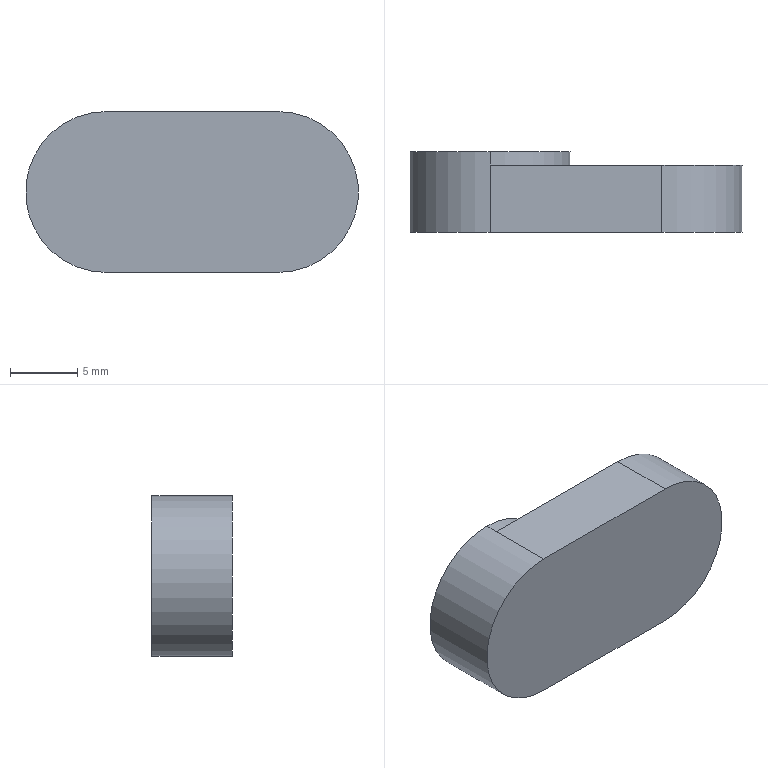Part | STEP file | JTJTRUYIU_Default | 1 solid | 8 faces | box 24.8 x 6 x 12 mm | volume 1447 mm3 | plane 5 | cylinder 3 | commonest cylinder face diameters 12 x3
STEP:
#1=CARTESIAN_POINT('',(0.,0.,0.));
#2=DIRECTION('',(0.,0.,1.));
#3=DIRECTION('',(1.,0.,0.));
#4=AXIS2_PLACEMENT_3D('',#1,#2,#3);
#5=CARTESIAN_POINT('',(-6.4,6.,6.));
#6=VERTEX_POINT('',#5);
#7=CARTESIAN_POINT('',(-6.4,6.,-6.));
#8=VERTEX_POINT('',#7);
#9=CARTESIAN_POINT('',(-6.4,6.,0.));
#10=DIRECTION('',(0.,1.,0.));
#11=DIRECTION('',(0.,0.,1.));
#12=AXIS2_PLACEMENT_3D('',#9,#10,#11);
#13=CIRCLE('',#12,6.);
#14=CARTESIAN_POINT('',(-6.4,5.,0.));
#15=DIRECTION('',(0.,-1.,0.));
#16=DIRECTION('',(0.,0.,-1.));
#17=AXIS2_PLACEMENT_3D('',#14,#15,#16);
#18=CYLINDRICAL_SURFACE('',#17,6.);
#19=CARTESIAN_POINT('',(3.142,-1.));
#20=DIRECTION('',(-1.,0.));
#21=VECTOR('',#20,1.);
#22=LINE('',#19,#21);
#23=(GEOMETRIC_REPRESENTATION_CONTEXT(2)PARAMETRIC_REPRESENTATION_CONTEXT()REPRESENTATION_CONTEXT('',''));
#24=DEFINITIONAL_REPRESENTATION('',(#22),#23);
#25=PCURVE('',#18,#24);
#26=CARTESIAN_POINT('',(-6.4,6.,0.));
#27=DIRECTION('',(0.,1.,0.));
#28=DIRECTION('',(0.,0.,1.));
#29=AXIS2_PLACEMENT_3D('',#26,#27,#28);
#30=PLANE('',#29);
#31=CARTESIAN_POINT('',(0.,0.));
#32=DIRECTION('',(1.,0.));
#33=AXIS2_PLACEMENT_2D('',#31,#32);
#34=CIRCLE('',#33,6.);
#35=(GEOMETRIC_REPRESENTATION_CONTEXT(2)PARAMETRIC_REPRESENTATION_CONTEXT()REPRESENTATION_CONTEXT('',''));
#36=DEFINITIONAL_REPRESENTATION('',(#34),#35);
#37=PCURVE('',#30,#36);
#38=SURFACE_CURVE('',#13,(#25,#37),.PCURVE_S1.);
#39=EDGE_CURVE('',#6,#8,#38,.T.);
#40=ORIENTED_EDGE('',*,*,#39,.F.);
#41=CARTESIAN_POINT('',(-6.4,5.,6.));
#42=VERTEX_POINT('',#41);
#43=CARTESIAN_POINT('',(-6.4,5.,6.));
#44=DIRECTION('',(0.,-1.,0.));
#45=VECTOR('',#44,1.);
#46=LINE('',#43,#45);
#47=CARTESIAN_POINT('',(3.142,0.));
#48=DIRECTION('',(0.,1.));
#49=VECTOR('',#48,1.);
#50=LINE('',#47,#49);
#51=(GEOMETRIC_REPRESENTATION_CONTEXT(2)PARAMETRIC_REPRESENTATION_CONTEXT()REPRESENTATION_CONTEXT('',''));
#52=DEFINITIONAL_REPRESENTATION('',(#50),#51);
#53=PCURVE('',#18,#52);
#54=CARTESIAN_POINT('',(-6.4,5.,0.));
#55=DIRECTION('',(0.,-1.,0.));
#56=DIRECTION('',(0.,0.,-1.));
#57=AXIS2_PLACEMENT_3D('',#54,#55,#56);
#58=CYLINDRICAL_SURFACE('',#57,6.);
#59=CARTESIAN_POINT('',(3.142,0.));
#60=DIRECTION('',(0.,1.));
#61=VECTOR('',#60,1.);
#62=LINE('',#59,#61);
#63=(GEOMETRIC_REPRESENTATION_CONTEXT(2)PARAMETRIC_REPRESENTATION_CONTEXT()REPRESENTATION_CONTEXT('',''));
#64=DEFINITIONAL_REPRESENTATION('',(#62),#63);
#65=PCURVE('',#58,#64);
#66=SURFACE_CURVE('',#46,(#53,#65),.PCURVE_S1.);
#67=EDGE_CURVE('',#6,#42,#66,.T.);
#68=ORIENTED_EDGE('',*,*,#67,.T.);
#69=CARTESIAN_POINT('',(-6.4,5.,-6.));
#70=VERTEX_POINT('',#69);
#71=CARTESIAN_POINT('',(-6.4,5.,0.));
#72=DIRECTION('',(0.,1.,0.));
#73=DIRECTION('',(0.,0.,1.));
#74=AXIS2_PLACEMENT_3D('',#71,#72,#73);
#75=CIRCLE('',#74,6.);
#76=CARTESIAN_POINT('',(3.142,0.));
#77=DIRECTION('',(-1.,0.));
#78=VECTOR('',#77,1.);
#79=LINE('',#76,#78);
#80=(GEOMETRIC_REPRESENTATION_CONTEXT(2)PARAMETRIC_REPRESENTATION_CONTEXT()REPRESENTATION_CONTEXT('',''));
#81=DEFINITIONAL_REPRESENTATION('',(#79),#80);
#82=PCURVE('',#18,#81);
#83=CARTESIAN_POINT('',(6.4,5.,0.));
#84=DIRECTION('',(0.,1.,0.));
#85=DIRECTION('',(0.,0.,1.));
#86=AXIS2_PLACEMENT_3D('',#83,#84,#85);
#87=PLANE('',#86);
#88=CARTESIAN_POINT('',(0.,-12.8));
#89=DIRECTION('',(1.,0.));
#90=AXIS2_PLACEMENT_2D('',#88,#89);
#91=CIRCLE('',#90,6.);
#92=(GEOMETRIC_REPRESENTATION_CONTEXT(2)PARAMETRIC_REPRESENTATION_CONTEXT()REPRESENTATION_CONTEXT('',''));
#93=DEFINITIONAL_REPRESENTATION('',(#91),#92);
#94=PCURVE('',#87,#93);
#95=SURFACE_CURVE('',#75,(#82,#94),.PCURVE_S1.);
#96=EDGE_CURVE('',#42,#70,#95,.T.);
#97=ORIENTED_EDGE('',*,*,#96,.T.);
#98=CARTESIAN_POINT('',(-6.4,5.,-6.));
#99=DIRECTION('',(0.,-1.,0.));
#100=VECTOR('',#99,1.);
#101=LINE('',#98,#100);
#102=CARTESIAN_POINT('',(0.,0.));
#103=DIRECTION('',(0.,1.));
#104=VECTOR('',#103,1.);
#105=LINE('',#102,#104);
#106=(GEOMETRIC_REPRESENTATION_CONTEXT(2)PARAMETRIC_REPRESENTATION_CONTEXT()REPRESENTATION_CONTEXT('',''));
#107=DEFINITIONAL_REPRESENTATION('',(#105),#106);
#108=PCURVE('',#18,#107);
#109=CARTESIAN_POINT('',(6.283,0.));
#110=DIRECTION('',(0.,1.));
#111=VECTOR('',#110,1.);
#112=LINE('',#109,#111);
#113=(GEOMETRIC_REPRESENTATION_CONTEXT(2)PARAMETRIC_REPRESENTATION_CONTEXT()REPRESENTATION_CONTEXT('',''));
#114=DEFINITIONAL_REPRESENTATION('',(#112),#113);
#115=PCURVE('',#58,#114);
#116=SURFACE_CURVE('',#101,(#108,#115),.PCURVE_S1.);
#117=EDGE_CURVE('',#8,#70,#116,.T.);
#118=ORIENTED_EDGE('',*,*,#117,.F.);
#119=EDGE_LOOP('',(#40,#68,#97,#118));
#120=FACE_BOUND('',#119,.T.);
#121=ADVANCED_FACE('',(#120),#18,.T.);
#122=CARTESIAN_POINT('',(6.4,0.,6.));
#123=VERTEX_POINT('',#122);
#124=CARTESIAN_POINT('',(6.4,0.,-6.));
#125=VERTEX_POINT('',#124);
#126=CARTESIAN_POINT('',(6.4,0.,0.));
#127=DIRECTION('',(0.,1.,0.));
#128=DIRECTION('',(0.,0.,1.));
#129=AXIS2_PLACEMENT_3D('',#126,#127,#128);
#130=CIRCLE('',#129,6.);
#131=CARTESIAN_POINT('',(6.4,5.,0.));
#132=DIRECTION('',(0.,-1.,0.));
#133=DIRECTION('',(0.,0.,-1.));
#134=AXIS2_PLACEMENT_3D('',#131,#132,#133);
#135=CYLINDRICAL_SURFACE('',#134,6.);
#136=CARTESIAN_POINT('',(3.142,5.));
#137=DIRECTION('',(-1.,0.));
#138=VECTOR('',#137,1.);
#139=LINE('',#136,#138);
#140=(GEOMETRIC_REPRESENTATION_CONTEXT(2)PARAMETRIC_REPRESENTATION_CONTEXT()REPRESENTATION_CONTEXT('',''));
#141=DEFINITIONAL_REPRESENTATION('',(#139),#140);
#142=PCURVE('',#135,#141);
#143=CARTESIAN_POINT('',(6.4,0.,0.));
#144=DIRECTION('',(0.,1.,0.));
#145=DIRECTION('',(0.,0.,1.));
#146=AXIS2_PLACEMENT_3D('',#143,#144,#145);
#147=PLANE('',#146);
#148=CARTESIAN_POINT('',(0.,0.));
#149=DIRECTION('',(1.,0.));
#150=AXIS2_PLACEMENT_2D('',#148,#149);
#151=CIRCLE('',#150,6.);
#152=(GEOMETRIC_REPRESENTATION_CONTEXT(2)PARAMETRIC_REPRESENTATION_CONTEXT()REPRESENTATION_CONTEXT('',''));
#153=DEFINITIONAL_REPRESENTATION('',(#151),#152);
#154=PCURVE('',#147,#153);
#155=SURFACE_CURVE('',#130,(#142,#154),.PCURVE_S1.);
#156=EDGE_CURVE('',#123,#125,#155,.T.);
#157=ORIENTED_EDGE('',*,*,#156,.T.);
#158=CARTESIAN_POINT('',(6.4,5.,-6.));
#159=VERTEX_POINT('',#158);
#160=CARTESIAN_POINT('',(6.4,5.,-6.));
#161=DIRECTION('',(0.,-1.,0.));
#162=VECTOR('',#161,1.);
#163=LINE('',#160,#162);
#164=CARTESIAN_POINT('',(0.,0.));
#165=DIRECTION('',(0.,1.));
#166=VECTOR('',#165,1.);
#167=LINE('',#164,#166);
#168=(GEOMETRIC_REPRESENTATION_CONTEXT(2)PARAMETRIC_REPRESENTATION_CONTEXT()REPRESENTATION_CONTEXT('',''));
#169=DEFINITIONAL_REPRESENTATION('',(#167),#168);
#170=PCURVE('',#135,#169);
#171=CARTESIAN_POINT('',(6.4,5.,-6.));
#172=DIRECTION('',(0.,0.,1.));
#173=DIRECTION('',(1.,0.,0.));
#174=AXIS2_PLACEMENT_3D('',#171,#172,#173);
#175=PLANE('',#174);
#176=CARTESIAN_POINT('',(0.,0.));
#177=DIRECTION('',(0.,-1.));
#178=VECTOR('',#177,1.);
#179=LINE('',#176,#178);
#180=(GEOMETRIC_REPRESENTATION_CONTEXT(2)PARAMETRIC_REPRESENTATION_CONTEXT()REPRESENTATION_CONTEXT('',''));
#181=DEFINITIONAL_REPRESENTATION('',(#179),#180);
#182=PCURVE('',#175,#181);
#183=SURFACE_CURVE('',#163,(#170,#182),.PCURVE_S1.);
#184=EDGE_CURVE('',#159,#125,#183,.T.);
#185=ORIENTED_EDGE('',*,*,#184,.F.);
#186=CARTESIAN_POINT('',(6.4,5.,6.));
#187=VERTEX_POINT('',#186);
#188=CARTESIAN_POINT('',(6.4,5.,0.));
#189=DIRECTION('',(0.,1.,0.));
#190=DIRECTION('',(0.,0.,1.));
#191=AXIS2_PLACEMENT_3D('',#188,#189,#190);
#192=CIRCLE('',#191,6.);
#193=CARTESIAN_POINT('',(3.142,0.));
#194=DIRECTION('',(-1.,0.));
#195=VECTOR('',#194,1.);
#196=LINE('',#193,#195);
#197=(GEOMETRIC_REPRESENTATION_CONTEXT(2)PARAMETRIC_REPRESENTATION_CONTEXT()REPRESENTATION_CONTEXT('',''));
#198=DEFINITIONAL_REPRESENTATION('',(#196),#197);
#199=PCURVE('',#135,#198);
#200=CARTESIAN_POINT('',(0.,0.));
#201=DIRECTION('',(1.,0.));
#202=AXIS2_PLACEMENT_2D('',#200,#201);
#203=CIRCLE('',#202,6.);
#204=(GEOMETRIC_REPRESENTATION_CONTEXT(2)PARAMETRIC_REPRESENTATION_CONTEXT()REPRESENTATION_CONTEXT('',''));
#205=DEFINITIONAL_REPRESENTATION('',(#203),#204);
#206=PCURVE('',#87,#205);
#207=SURFACE_CURVE('',#192,(#199,#206),.PCURVE_S1.);
#208=EDGE_CURVE('',#187,#159,#207,.T.);
#209=ORIENTED_EDGE('',*,*,#208,.F.);
#210=CARTESIAN_POINT('',(6.4,5.,6.));
#211=DIRECTION('',(0.,-1.,0.));
#212=VECTOR('',#211,1.);
#213=LINE('',#210,#212);
#214=CARTESIAN_POINT('',(3.142,0.));
#215=DIRECTION('',(0.,1.));
#216=VECTOR('',#215,1.);
#217=LINE('',#214,#216);
#218=(GEOMETRIC_REPRESENTATION_CONTEXT(2)PARAMETRIC_REPRESENTATION_CONTEXT()REPRESENTATION_CONTEXT('',''));
#219=DEFINITIONAL_REPRESENTATION('',(#217),#218);
#220=PCURVE('',#135,#219);
#221=CARTESIAN_POINT('',(6.4,5.,6.));
#222=DIRECTION('',(0.,0.,-1.));
#223=DIRECTION('',(-1.,0.,0.));
#224=AXIS2_PLACEMENT_3D('',#221,#222,#223);
#225=PLANE('',#224);
#226=CARTESIAN_POINT('',(0.,0.));
#227=DIRECTION('',(0.,-1.));
#228=VECTOR('',#227,1.);
#229=LINE('',#226,#228);
#230=(GEOMETRIC_REPRESENTATION_CONTEXT(2)PARAMETRIC_REPRESENTATION_CONTEXT()REPRESENTATION_CONTEXT('',''));
#231=DEFINITIONAL_REPRESENTATION('',(#229),#230);
#232=PCURVE('',#225,#231);
#233=SURFACE_CURVE('',#213,(#220,#232),.PCURVE_S1.);
#234=EDGE_CURVE('',#187,#123,#233,.T.);
#235=ORIENTED_EDGE('',*,*,#234,.T.);
#236=EDGE_LOOP('',(#157,#185,#209,#235));
#237=FACE_BOUND('',#236,.T.);
#238=ADVANCED_FACE('',(#237),#135,.T.);
#239=CARTESIAN_POINT('',(-6.4,0.,-6.));
#240=VERTEX_POINT('',#239);
#241=CARTESIAN_POINT('',(6.4,0.,-6.));
#242=DIRECTION('',(-1.,0.,0.));
#243=VECTOR('',#242,1.);
#244=LINE('',#241,#243);
#245=CARTESIAN_POINT('',(0.,-5.));
#246=DIRECTION('',(-1.,0.));
#247=VECTOR('',#246,1.);
#248=LINE('',#245,#247);
#249=(GEOMETRIC_REPRESENTATION_CONTEXT(2)PARAMETRIC_REPRESENTATION_CONTEXT()REPRESENTATION_CONTEXT('',''));
#250=DEFINITIONAL_REPRESENTATION('',(#248),#249);
#251=PCURVE('',#175,#250);
#252=CARTESIAN_POINT('',(-6.,0.));
#253=DIRECTION('',(0.,-1.));
#254=VECTOR('',#253,1.);
#255=LINE('',#252,#254);
#256=(GEOMETRIC_REPRESENTATION_CONTEXT(2)PARAMETRIC_REPRESENTATION_CONTEXT()REPRESENTATION_CONTEXT('',''));
#257=DEFINITIONAL_REPRESENTATION('',(#255),#256);
#258=PCURVE('',#147,#257);
#259=SURFACE_CURVE('',#244,(#251,#258),.PCURVE_S1.);
#260=EDGE_CURVE('',#125,#240,#259,.T.);
#261=ORIENTED_EDGE('',*,*,#260,.T.);
#262=CARTESIAN_POINT('',(-6.4,5.,-6.));
#263=DIRECTION('',(0.,-1.,0.));
#264=VECTOR('',#263,1.);
#265=LINE('',#262,#264);
#266=CARTESIAN_POINT('',(-12.8,0.));
#267=DIRECTION('',(0.,-1.));
#268=VECTOR('',#267,1.);
#269=LINE('',#266,#268);
#270=(GEOMETRIC_REPRESENTATION_CONTEXT(2)PARAMETRIC_REPRESENTATION_CONTEXT()REPRESENTATION_CONTEXT('',''));
#271=DEFINITIONAL_REPRESENTATION('',(#269),#270);
#272=PCURVE('',#175,#271);
#273=CARTESIAN_POINT('',(6.283,0.));
#274=DIRECTION('',(0.,1.));
#275=VECTOR('',#274,1.);
#276=LINE('',#273,#275);
#277=(GEOMETRIC_REPRESENTATION_CONTEXT(2)PARAMETRIC_REPRESENTATION_CONTEXT()REPRESENTATION_CONTEXT('',''));
#278=DEFINITIONAL_REPRESENTATION('',(#276),#277);
#279=PCURVE('',#58,#278);
#280=SURFACE_CURVE('',#265,(#272,#279),.PCURVE_S1.);
#281=EDGE_CURVE('',#70,#240,#280,.T.);
#282=ORIENTED_EDGE('',*,*,#281,.F.);
#283=CARTESIAN_POINT('',(6.4,5.,-6.));
#284=DIRECTION('',(-1.,0.,0.));
#285=VECTOR('',#284,1.);
#286=LINE('',#283,#285);
#287=CARTESIAN_POINT('',(0.,0.));
#288=DIRECTION('',(-1.,0.));
#289=VECTOR('',#288,1.);
#290=LINE('',#287,#289);
#291=(GEOMETRIC_REPRESENTATION_CONTEXT(2)PARAMETRIC_REPRESENTATION_CONTEXT()REPRESENTATION_CONTEXT('',''));
#292=DEFINITIONAL_REPRESENTATION('',(#290),#291);
#293=PCURVE('',#175,#292);
#294=CARTESIAN_POINT('',(-6.,0.));
#295=DIRECTION('',(0.,-1.));
#296=VECTOR('',#295,1.);
#297=LINE('',#294,#296);
#298=(GEOMETRIC_REPRESENTATION_CONTEXT(2)PARAMETRIC_REPRESENTATION_CONTEXT()REPRESENTATION_CONTEXT('',''));
#299=DEFINITIONAL_REPRESENTATION('',(#297),#298);
#300=PCURVE('',#87,#299);
#301=SURFACE_CURVE('',#286,(#293,#300),.PCURVE_S1.);
#302=EDGE_CURVE('',#159,#70,#301,.T.);
#303=ORIENTED_EDGE('',*,*,#302,.F.);
#304=ORIENTED_EDGE('',*,*,#184,.T.);
#305=EDGE_LOOP('',(#261,#282,#303,#304));
#306=FACE_BOUND('',#305,.T.);
#307=ADVANCED_FACE('',(#306),#175,.F.);
#308=ORIENTED_EDGE('',*,*,#67,.F.);
#309=CARTESIAN_POINT('',(-6.4,6.,0.));
#310=DIRECTION('',(0.,1.,0.));
#311=DIRECTION('',(0.,0.,1.));
#312=AXIS2_PLACEMENT_3D('',#309,#310,#311);
#313=CIRCLE('',#312,6.);
#314=CARTESIAN_POINT('',(9.425,-1.));
#315=DIRECTION('',(-1.,0.));
#316=VECTOR('',#315,1.);
#317=LINE('',#314,#316);
#318=(GEOMETRIC_REPRESENTATION_CONTEXT(2)PARAMETRIC_REPRESENTATION_CONTEXT()REPRESENTATION_CONTEXT('',''));
#319=DEFINITIONAL_REPRESENTATION('',(#317),#318);
#320=PCURVE('',#58,#319);
#321=CARTESIAN_POINT('',(0.,0.));
#322=DIRECTION('',(1.,0.));
#323=AXIS2_PLACEMENT_2D('',#321,#322);
#324=CIRCLE('',#323,6.);
#325=(GEOMETRIC_REPRESENTATION_CONTEXT(2)PARAMETRIC_REPRESENTATION_CONTEXT()REPRESENTATION_CONTEXT('',''));
#326=DEFINITIONAL_REPRESENTATION('',(#324),#325);
#327=PCURVE('',#30,#326);
#328=SURFACE_CURVE('',#313,(#320,#327),.PCURVE_S1.);
#329=EDGE_CURVE('',#8,#6,#328,.T.);
#330=ORIENTED_EDGE('',*,*,#329,.F.);
#331=ORIENTED_EDGE('',*,*,#117,.T.);
#332=ORIENTED_EDGE('',*,*,#281,.T.);
#333=CARTESIAN_POINT('',(-6.4,0.,6.));
#334=VERTEX_POINT('',#333);
#335=CARTESIAN_POINT('',(-6.4,0.,0.));
#336=DIRECTION('',(0.,1.,0.));
#337=DIRECTION('',(0.,0.,1.));
#338=AXIS2_PLACEMENT_3D('',#335,#336,#337);
#339=CIRCLE('',#338,6.);
#340=CARTESIAN_POINT('',(9.425,5.));
#341=DIRECTION('',(-1.,0.));
#342=VECTOR('',#341,1.);
#343=LINE('',#340,#342);
#344=(GEOMETRIC_REPRESENTATION_CONTEXT(2)PARAMETRIC_REPRESENTATION_CONTEXT()REPRESENTATION_CONTEXT('',''));
#345=DEFINITIONAL_REPRESENTATION('',(#343),#344);
#346=PCURVE('',#58,#345);
#347=CARTESIAN_POINT('',(0.,-12.8));
#348=DIRECTION('',(1.,0.));
#349=AXIS2_PLACEMENT_2D('',#347,#348);
#350=CIRCLE('',#349,6.);
#351=(GEOMETRIC_REPRESENTATION_CONTEXT(2)PARAMETRIC_REPRESENTATION_CONTEXT()REPRESENTATION_CONTEXT('',''));
#352=DEFINITIONAL_REPRESENTATION('',(#350),#351);
#353=PCURVE('',#147,#352);
#354=SURFACE_CURVE('',#339,(#346,#353),.PCURVE_S1.);
#355=EDGE_CURVE('',#240,#334,#354,.T.);
#356=ORIENTED_EDGE('',*,*,#355,.T.);
#357=CARTESIAN_POINT('',(-6.4,5.,6.));
#358=DIRECTION('',(0.,-1.,0.));
#359=VECTOR('',#358,1.);
#360=LINE('',#357,#359);
#361=CARTESIAN_POINT('',(3.142,0.));
#362=DIRECTION('',(0.,1.));
#363=VECTOR('',#362,1.);
#364=LINE('',#361,#363);
#365=(GEOMETRIC_REPRESENTATION_CONTEXT(2)PARAMETRIC_REPRESENTATION_CONTEXT()REPRESENTATION_CONTEXT('',''));
#366=DEFINITIONAL_REPRESENTATION('',(#364),#365);
#367=PCURVE('',#58,#366);
#368=CARTESIAN_POINT('',(12.8,0.));
#369=DIRECTION('',(0.,-1.));
#370=VECTOR('',#369,1.);
#371=LINE('',#368,#370);
#372=(GEOMETRIC_REPRESENTATION_CONTEXT(2)PARAMETRIC_REPRESENTATION_CONTEXT()REPRESENTATION_CONTEXT('',''));
#373=DEFINITIONAL_REPRESENTATION('',(#371),#372);
#374=PCURVE('',#225,#373);
#375=SURFACE_CURVE('',#360,(#367,#374),.PCURVE_S1.);
#376=EDGE_CURVE('',#42,#334,#375,.T.);
#377=ORIENTED_EDGE('',*,*,#376,.F.);
#378=EDGE_LOOP('',(#308,#330,#331,#332,#356,#377));
#379=FACE_BOUND('',#378,.T.);
#380=ADVANCED_FACE('',(#379),#58,.T.);
#381=CARTESIAN_POINT('',(6.4,0.,6.));
#382=DIRECTION('',(1.,0.,0.));
#383=VECTOR('',#382,1.);
#384=LINE('',#381,#383);
#385=CARTESIAN_POINT('',(0.,-5.));
#386=DIRECTION('',(-1.,0.));
#387=VECTOR('',#386,1.);
#388=LINE('',#385,#387);
#389=(GEOMETRIC_REPRESENTATION_CONTEXT(2)PARAMETRIC_REPRESENTATION_CONTEXT()REPRESENTATION_CONTEXT('',''));
#390=DEFINITIONAL_REPRESENTATION('',(#388),#389);
#391=PCURVE('',#225,#390);
#392=CARTESIAN_POINT('',(6.,0.));
#393=DIRECTION('',(0.,1.));
#394=VECTOR('',#393,1.);
#395=LINE('',#392,#394);
#396=(GEOMETRIC_REPRESENTATION_CONTEXT(2)PARAMETRIC_REPRESENTATION_CONTEXT()REPRESENTATION_CONTEXT('',''));
#397=DEFINITIONAL_REPRESENTATION('',(#395),#396);
#398=PCURVE('',#147,#397);
#399=SURFACE_CURVE('',#384,(#391,#398),.PCURVE_S1.);
#400=EDGE_CURVE('',#334,#123,#399,.T.);
#401=ORIENTED_EDGE('',*,*,#400,.T.);
#402=ORIENTED_EDGE('',*,*,#234,.F.);
#403=CARTESIAN_POINT('',(6.4,5.,6.));
#404=DIRECTION('',(1.,0.,0.));
#405=VECTOR('',#404,1.);
#406=LINE('',#403,#405);
#407=CARTESIAN_POINT('',(0.,0.));
#408=DIRECTION('',(-1.,0.));
#409=VECTOR('',#408,1.);
#410=LINE('',#407,#409);
#411=(GEOMETRIC_REPRESENTATION_CONTEXT(2)PARAMETRIC_REPRESENTATION_CONTEXT()REPRESENTATION_CONTEXT('',''));
#412=DEFINITIONAL_REPRESENTATION('',(#410),#411);
#413=PCURVE('',#225,#412);
#414=CARTESIAN_POINT('',(6.,0.));
#415=DIRECTION('',(0.,1.));
#416=VECTOR('',#415,1.);
#417=LINE('',#414,#416);
#418=(GEOMETRIC_REPRESENTATION_CONTEXT(2)PARAMETRIC_REPRESENTATION_CONTEXT()REPRESENTATION_CONTEXT('',''));
#419=DEFINITIONAL_REPRESENTATION('',(#417),#418);
#420=PCURVE('',#87,#419);
#421=SURFACE_CURVE('',#406,(#413,#420),.PCURVE_S1.);
#422=EDGE_CURVE('',#42,#187,#421,.T.);
#423=ORIENTED_EDGE('',*,*,#422,.F.);
#424=ORIENTED_EDGE('',*,*,#376,.T.);
#425=EDGE_LOOP('',(#401,#402,#423,#424));
#426=FACE_BOUND('',#425,.T.);
#427=ADVANCED_FACE('',(#426),#225,.F.);
#428=ORIENTED_EDGE('',*,*,#96,.F.);
#429=ORIENTED_EDGE('',*,*,#422,.T.);
#430=ORIENTED_EDGE('',*,*,#208,.T.);
#431=ORIENTED_EDGE('',*,*,#302,.T.);
#432=EDGE_LOOP('',(#428,#429,#430,#431));
#433=FACE_BOUND('',#432,.T.);
#434=ADVANCED_FACE('',(#433),#87,.T.);
#435=ORIENTED_EDGE('',*,*,#156,.F.);
#436=ORIENTED_EDGE('',*,*,#400,.F.);
#437=ORIENTED_EDGE('',*,*,#355,.F.);
#438=ORIENTED_EDGE('',*,*,#260,.F.);
#439=EDGE_LOOP('',(#435,#436,#437,#438));
#440=FACE_BOUND('',#439,.T.);
#441=ADVANCED_FACE('',(#440),#147,.F.);
#442=ORIENTED_EDGE('',*,*,#329,.T.);
#443=ORIENTED_EDGE('',*,*,#39,.T.);
#444=EDGE_LOOP('',(#442,#443));
#445=FACE_BOUND('',#444,.T.);
#446=ADVANCED_FACE('',(#445),#30,.T.);
#447=CLOSED_SHELL('',(#121,#238,#307,#380,#427,#434,#441,#446));
#448=MANIFOLD_SOLID_BREP('',#447);
#449=(LENGTH_UNIT()NAMED_UNIT(*)SI_UNIT(.MILLI.,.METRE.));
#450=UNCERTAINTY_MEASURE_WITH_UNIT(LENGTH_MEASURE(0.0000001),#449,'','');
#451=(NAMED_UNIT(*)PLANE_ANGLE_UNIT()SI_UNIT($,.RADIAN.));
#452=(NAMED_UNIT(*)SI_UNIT($,.STERADIAN.)SOLID_ANGLE_UNIT());
#453=(GEOMETRIC_REPRESENTATION_CONTEXT(3)GLOBAL_UNCERTAINTY_ASSIGNED_CONTEXT((#450))GLOBAL_UNIT_ASSIGNED_CONTEXT((#449,#451,#452))REPRESENTATION_CONTEXT('',''));
#454=ADVANCED_BREP_SHAPE_REPRESENTATION('',(#4,#448),#453);